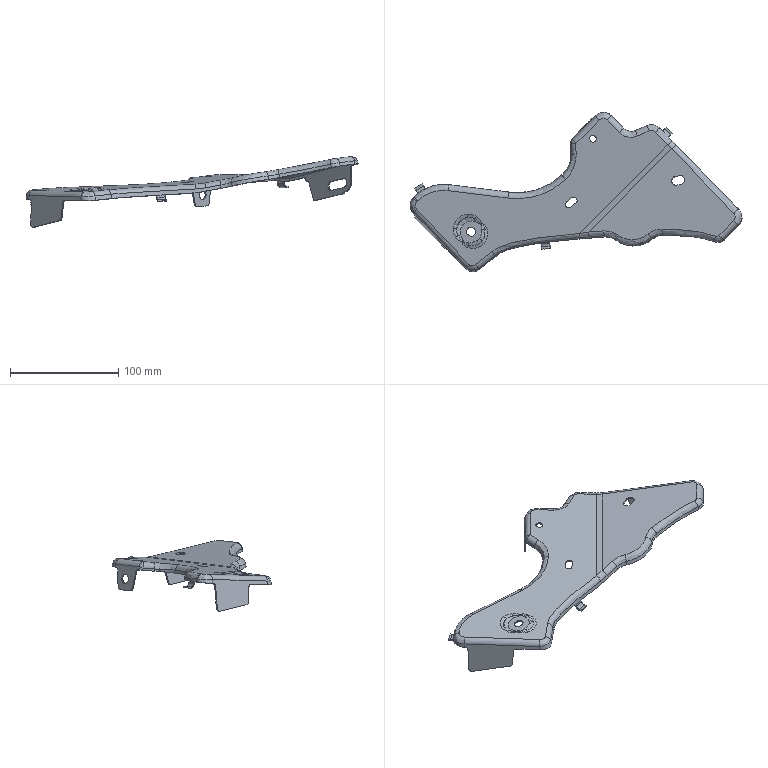Part | STEP file | PN_0003_id646_x_t | 1 solid | 286 faces | box 307.193 x 147.409 x 65.496 mm | volume 34303 mm3 | spline 201 | cylinder 42 | plane 36 | other 5 | sphere 2 | commonest cylinder face diameters 7.5 x10 10 x10 20 x6 17.5 x5 6 x3 8.2 x2